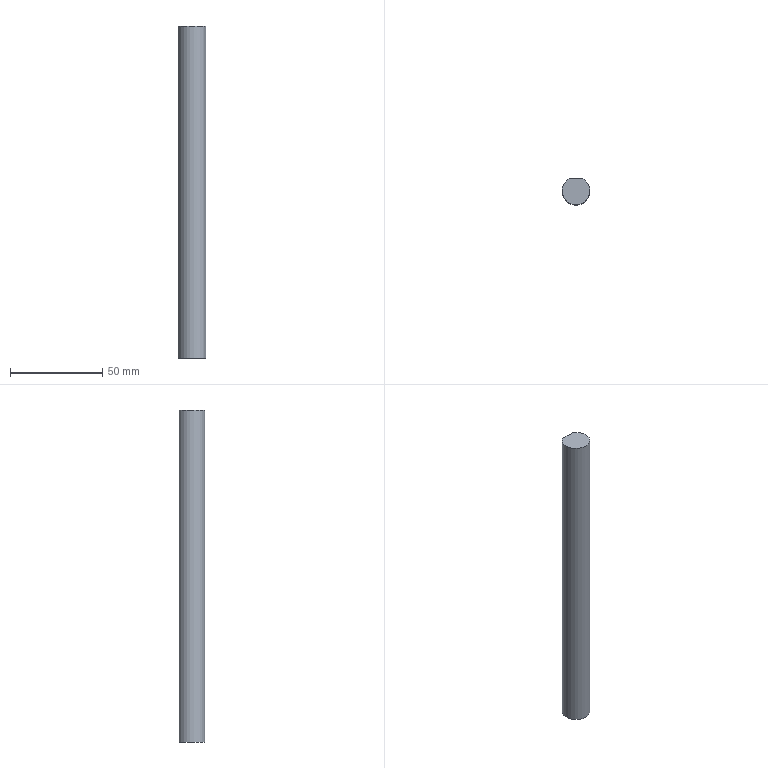CAM job | NX | 3+2 milling, drilling | part box 15 x 14 x 180 mm | stock box 15 x 15 x 180 mm
Tools:
number,name,description,diameter,corner_radius,flute_length,length,flutes
1,ZXZ,Milling Tool-5 Parameters,6.0,0.0,50.0,75.0,2
7,D6A45,Milling Tool-5 Parameters,6.0,0.0,3.0,3.0,2
3,3.3ZT,Drilling Tool,3.3,0.0,35.0,50.0,2
4,D16R0.8,Milling Tool-5 Parameters,16.0,0.8,50.0,75.0,2
Operations:
program,operation,operation_type,tool,method,geometry_group,spindle_rpm,surface_speed,feed_per_tooth,feed_cut,feed_plunge,cut_length_mm,path_length_mm,cut_time_min,machine_time_min
1,FLOOR_WALL,VolumeBased25DMillingOperation,D16R0.8,METHOD,A,2500.0,125.0,0.36,1800.0,100.0,1040.0,2124.001,0.5778,0.6862
1,DRILLING,Operation,ZXZ,METHOD,A,3000.0,56.0,0.0333,200.0,0.0,12.0,212.15,0.06,0.08
1,DRILLING_COPY,Operation,3.3ZT,METHOD,A,2000.0,20.0,0.03,120.0,0.0,42.274,272.698,0.3523,0.3753
1,DRILLING_COPY_1,Operation,D6A45,METHOD,A,3000.0,56.0,0.0333,200.0,0.0,15.0,218.15,0.075,0.0953
PROGRAM_COPY,ZLEVEL_PROFILE_1_COPY_1,ZLevelMilling,D6A45,METHOD,A,7500.0,141.0,0.0667,1000.0,100.0,0.0,0.0,0.0,0.0,missing